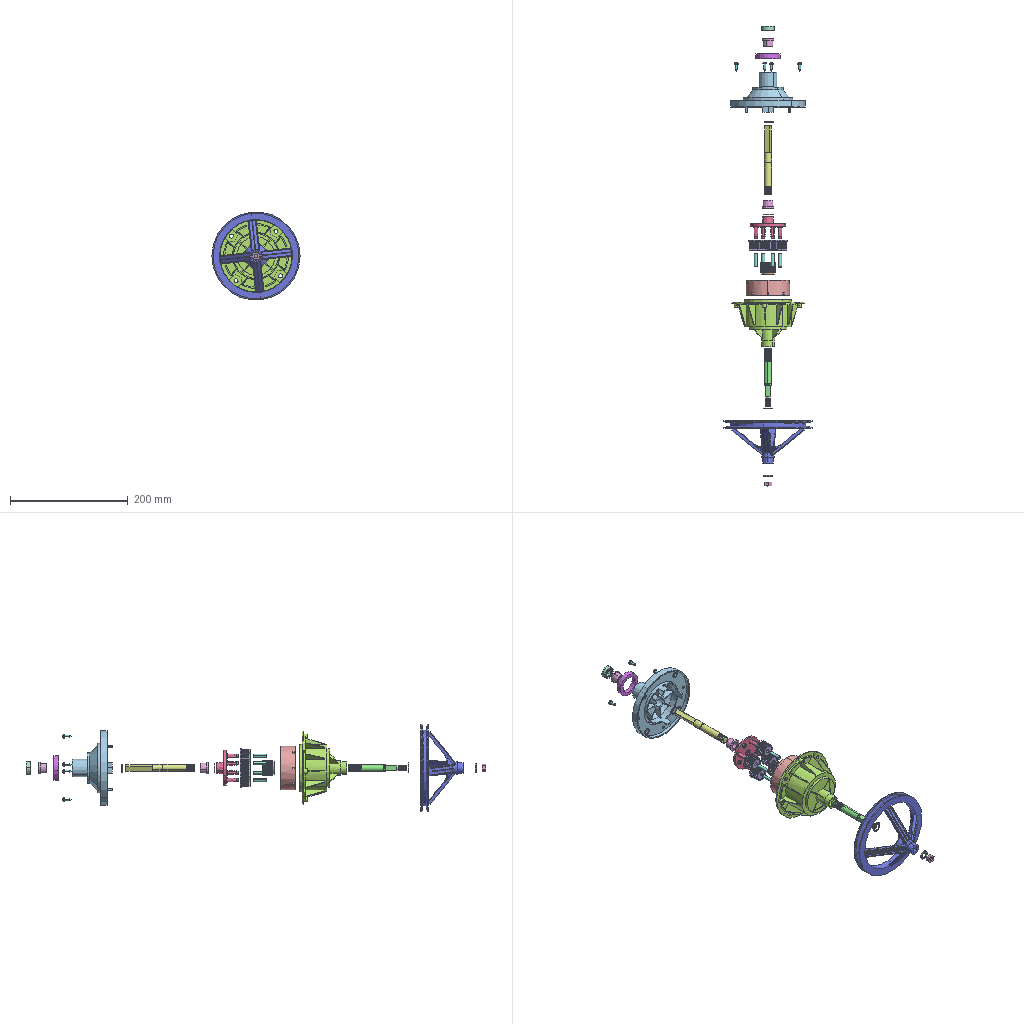Assembly | SolidWorks | 18 different items | 32 placed | box 150 x 782 x 149 mm
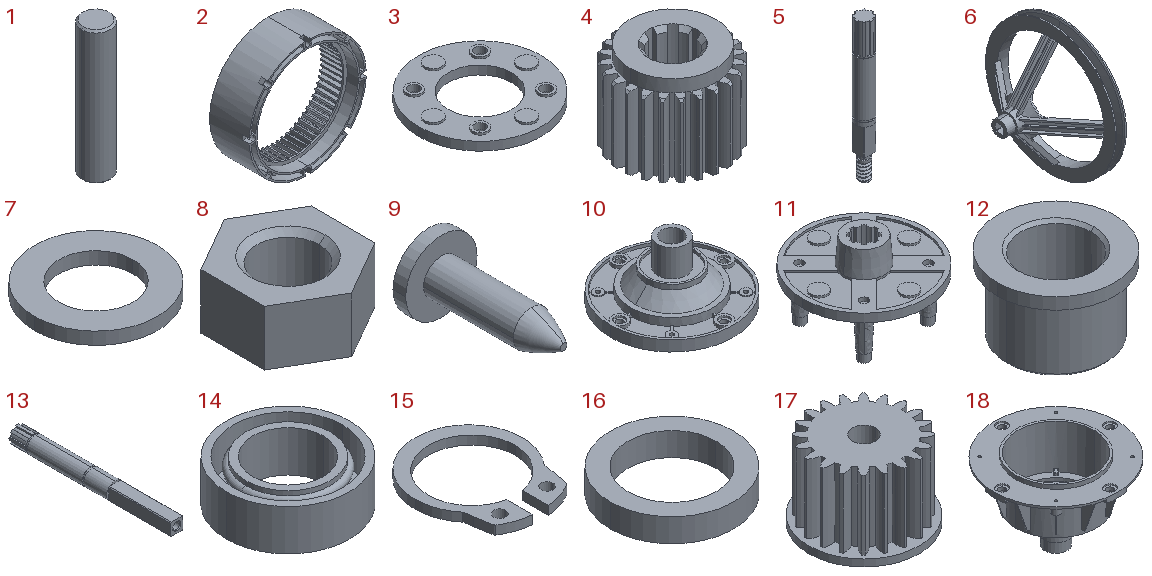Parts list (item | quantity | size | volume | features):
1 | x4 | 5 x 5 x 23 mm | 450.247 mm3 | features Chamfer 1, Extrusion 1
2 | x1 | 74 x 25 x 74 mm | 22545 mm3 | features ICE 6, CirPattern 1, Extrusion 1
3 | x1 | 58 x 58 x 5 mm | 7199 mm3 | features ICE 6, CirPattern 2, Extrusion 1
4 | x1 | 25.844 x 25.844 x 21 mm | 6942 mm3 | features Chamfer 3, ICE 2, Extrusion 1
5 | x1 | 12 x 12 x 100 mm | 8949 mm3 | features ICE 7, Chamfer 1, Extrusion 1, SweepThread 1
6 | x1 | 72 x 150 x 150 mm | 52845 mm3 | features ICE 6, CirPattern 2, Fillet 1, MirrorPattern 1, Revolution 1
7 | x1 | 15 x 15 x 1.5 mm | 169.646 mm3 | features Extrusion 1
8 | x1 | 12 x 13.856 x 6 mm | 525.917 mm3 | features Extrusion 1, HoleWzd 1
9 | x4 | 7 x 14.345 x 7 mm | 163.247 mm3 | features ICE 2, Revolution 2, CirPattern 1
10 | x1 | 127 x 127 x 68 mm | 67488 mm3 | features ICE 14, CirPattern 4, Extrusion 1, RevCut 1, Revolution 1
11 | x1 | 60 x 60 x 37 mm | 14280 mm3 | features ICE 8, CirPattern 5, Blend 1, Extrusion 1, Revolution 1
12 | x4 | 20 x 20 x 13 mm | 1639 mm3 | features ICE 2, Chamfer 1, Extrusion 1
13 | x1 | 12 x 116 x 12 mm | 11161 mm3 | features ICE 5, Extrusion 1, HoleWzd 1
14 | x1 | 21 x 21 x 7 mm | 1076 mm3 | features Extrusion 1, ICE 1, Revolution 1
15 | x3 | 13.6 x 15.943 x 1.1 mm | 71.659 mm3 | features Extrusion 1
16 | x1 | 42 x 42 x 8 mm | 5429 mm3 | features Extrusion 1
17 | x4 | 24 x 24 x 16.5 mm | 4627 mm3 | features ICE 3, Extrusion 1
18 | x1 | 123 x 123 x 80 mm | 67941 mm3 | features ICE 19, CirPattern 5, Rib 3, Extrusion 1, Fillet 1, MirrorPattern 1
Mates (type | each side: item.copy, entity, surface, feature):
Concentric | 2.1 edge | 18.1 edge
Coincident | 2.1 face plane Cut-Extrude6 | 18.1 face plane CirPattern7
Concentric | 3.1 face cylinder Boss-Extrude1 | 18.1 face cylinder Cut-Extrude1
Coincident | 3.1 face plane CirPattern1 | 18.1 face plane Cut-Extrude2
Concentric | 18.1 face cylinder Cut-Extrude3 | 12.1 face cylinder Cut-Extrude1
Coincident | 18.1 face plane Cut-Extrude1 | 12.1 face plane Boss-Extrude2
Concentric | 12.1 face cylinder Cut-Extrude1 | 5.1 face cylinder Boss-Extrude1
Concentric | 12.1 face cylinder Cut-Extrude1 | 4.1 edge
Coincident | 4.1 face plane Cut-Extrude1 | 5.1 face plane Boss-Extrude3
Coincident | 4.1 face plane Boss-Extrude2 | 5.1 face plane Boss-Extrude3
Concentric | 3.1 face cylinder Cut-Extrude4 | 1.1 face cylinder Boss-Extrude1
Coincident | 18.1 face plane Cut-Extrude2 | 1.1 face plane Boss-Extrude1
Concentric | 3.1 face cylinder CirPattern2 | 1.2 face cylinder Boss-Extrude1
Coincident | 18.1 face plane Cut-Extrude2 | 1.2 edge
Concentric | 3.1 face cylinder CirPattern2 | 1.3 face cylinder Boss-Extrude1
Coincident | 18.1 face plane Cut-Extrude2 | 1.3 face plane Boss-Extrude1
Concentric | 3.1 face cylinder CirPattern2 | 1.4 face cylinder Boss-Extrude1
Coincident | 18.1 face plane Cut-Extrude2 | 1.4 face plane Boss-Extrude1
Concentric | 1.4 face cylinder Boss-Extrude1 | 17.1 face cylinder Cut-Extrude1
Concentric | 1.3 face cylinder Boss-Extrude1 | 17.2 face cylinder Cut-Extrude1
Concentric | 1.2 face cylinder Boss-Extrude1 | 17.3 face cylinder Cut-Extrude1
Concentric | 1.1 face cylinder Boss-Extrude1 | 17.4 face cylinder Cut-Extrude1
Coincident | 4.1 face plane Boss-Extrude1 | 17.2 face plane Boss-Extrude1
Coincident | 4.1 face plane Boss-Extrude1 | 17.3 face plane Boss-Extrude1
Coincident | 4.1 face plane Boss-Extrude1 | 17.1 face plane Boss-Extrude1
Coincident | 4.1 face plane Boss-Extrude1 | 17.4 face plane Boss-Extrude1
Coincident | 12.1 face plane Boss-Extrude1 | 4.1 face plane Boss-Extrude2
Concentric | 18.1 face cylinder Cut-Extrude1 | 11.1 edge
Concentric | 17.2 face cylinder Cut-Extrude1 | 11.1 face cylinder CirPattern4
Coincident | 17.2 face plane Boss-Extrude1 | 11.1 face plane Boss-Extrude1
Coincident | 13.1 face plane Boss-Extrude1 | 15.1 face plane Boss-Extrude1
Concentric | 13.1 face cylinder Boss-Extrude5 | 15.1 edge
Concentric | 13.1 edge | 15.2 face cylinder Boss-Extrude1
Coincident | 13.1 face plane Boss-Extrude1 | 15.2 face plane Boss-Extrude1
Concentric | 11.1 edge | 13.1 face cylinder Boss-Extrude1
Coincident | 11.1 face plane Cut-Extrude5 | 13.1 face plane Boss-Extrude4
Coincident | 11.1 face plane Revolve1 | 15.2 face plane Boss-Extrude1
Concentric | 10.1 face cylinder Cut-Extrude4 | 12.2 face cylinder Boss-Extrude1
Coincident | 10.1 face plane Boss-Extrude3 | 12.2 face plane Boss-Extrude2
Concentric | 18.1 edge | 10.1 edge | 2 times
Coincident | 18.1 face plane Cut-Extrude7 | 10.1 face plane Boss-Extrude4
Concentric | 13.1 face cylinder Boss-Extrude6 | 12.3 face cylinder Boss-Extrude1
Concentric | 10.1 face cylinder Boss-Extrude1 | 16.1 face cylinder Boss-Extrude1
Coincident | 10.1 face plane Revolve1 | 16.1 face plane Boss-Extrude1
Concentric | 10.1 face cylinder Boss-Extrude1 | 14.1 face cylinder Boss-Extrude1
Coincident | 12.3 face plane Boss-Extrude1 | 14.1 face plane Boss-Extrude1
Concentric | 18.1 face cylinder Boss-Extrude4 | 12.4 face cylinder Boss-Extrude1
Coincident | 18.1 face plane Boss-Extrude4 | 12.4 face plane Boss-Extrude2
Concentric | 5.1 face cylinder Boss-Extrude4 | 15.3 face cylinder Boss-Extrude1
Coincident | 12.4 face plane Boss-Extrude1 | 15.3 face plane Boss-Extrude1
Concentric | 18.1 edge | 6.1 edge
Parallel | 5.1 face plane Boss-Extrude6 | 6.1 face plane Cut-Extrude3
Coincident | 5.1 face plane Boss-Extrude5 | 6.1 face plane Revolve1
Concentric | 6.1 edge | 7.1 edge
Coincident | 6.1 face plane Revolve1 | 7.1 edge
Concentric | 7.1 face cylinder Boss-Extrude1 | 8.1 edge
Coincident | 7.1 face plane Boss-Extrude1 | 8.1 face plane Boss-Extrude1
Concentric | 10.1 edge | 9.1 face cylinder Boss-Extrude1
Coincident | 10.1 face plane Cut-Extrude7 | 9.1 face plane Revolve2
Concentric | 10.1 face cylinder CirPattern2 | 9.2 face cylinder Boss-Extrude1
Coincident | 10.1 face plane CirPattern2 | 9.2 face plane Revolve2
Concentric | 10.1 face cylinder CirPattern2 | 9.3 face cylinder Boss-Extrude1
Coincident | 10.1 face plane CirPattern2 | 9.3 face plane Revolve2
Concentric | 10.1 face cylinder CirPattern2 | 9.4 face cylinder Boss-Extrude1
Coincident | 10.1 face plane CirPattern2 | 9.4 face plane Revolve2